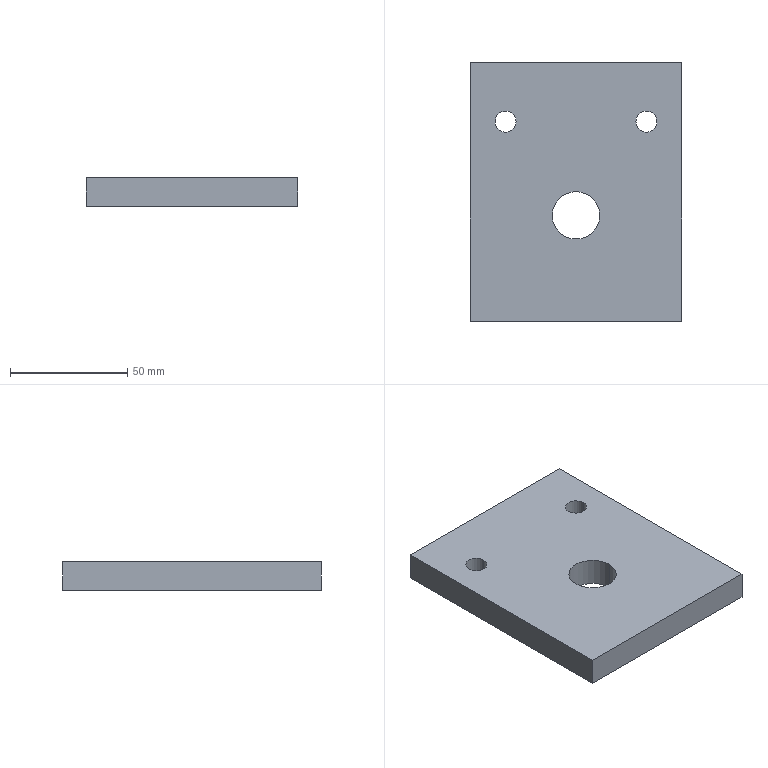Part | SolidWorks | features Extrusion 1, ICE 1 | 1 solid | 12 faces | box 90 x 110 x 12 mm | volume 113427 mm3 | cylinder 6 | plane 6 | commonest cylinder face diameters 9 x4 20.2 x2
STEP:
#1=CARTESIAN_POINT('',(-34.5,30.,-6.));
#2=VERTEX_POINT('',#1);
#3=CARTESIAN_POINT('',(-25.5,30.,-6.));
#4=VERTEX_POINT('',#3);
#5=CARTESIAN_POINT('',(-30.,30.,-6.));
#6=DIRECTION('',(0.,0.,1.));
#7=DIRECTION('',(1.,0.,0.));
#8=AXIS2_PLACEMENT_3D('',#5,#6,#7);
#9=CIRCLE('',#8,4.5);
#10=EDGE_CURVE('',#2,#4,#9,.T.);
#11=ORIENTED_EDGE('',*,*,#10,.F.);
#12=CARTESIAN_POINT('',(-34.5,30.,6.));
#13=VERTEX_POINT('',#12);
#14=CARTESIAN_POINT('',(-34.5,30.,-16.));
#15=DIRECTION('',(0.,0.,1.));
#16=VECTOR('',#15,1000.);
#17=LINE('',#14,#16);
#18=EDGE_CURVE('',#2,#13,#17,.T.);
#19=ORIENTED_EDGE('',*,*,#18,.T.);
#20=CARTESIAN_POINT('',(-25.5,30.,6.));
#21=VERTEX_POINT('',#20);
#22=CARTESIAN_POINT('',(-30.,30.,6.));
#23=DIRECTION('',(0.,0.,1.));
#24=DIRECTION('',(1.,0.,0.));
#25=AXIS2_PLACEMENT_3D('',#22,#23,#24);
#26=CIRCLE('',#25,4.5);
#27=EDGE_CURVE('',#13,#21,#26,.T.);
#28=ORIENTED_EDGE('',*,*,#27,.T.);
#29=CARTESIAN_POINT('',(-25.5,30.,-16.));
#30=DIRECTION('',(0.,0.,1.));
#31=VECTOR('',#30,1000.);
#32=LINE('',#29,#31);
#33=EDGE_CURVE('',#4,#21,#32,.T.);
#34=ORIENTED_EDGE('',*,*,#33,.F.);
#35=EDGE_LOOP('',(#11,#19,#28,#34));
#36=FACE_OUTER_BOUND('',#35,.T.);
#37=CARTESIAN_POINT('',(-30.,30.,-16.));
#38=DIRECTION('',(0.,0.,1.));
#39=DIRECTION('',(1.,0.,0.));
#40=AXIS2_PLACEMENT_3D('',#37,#38,#39);
#41=CYLINDRICAL_SURFACE('',#40,4.5);
#42=ADVANCED_FACE('',(#36),#41,.F.);
#43=CARTESIAN_POINT('',(25.5,30.,-6.));
#44=VERTEX_POINT('',#43);
#45=CARTESIAN_POINT('',(34.5,30.,-6.));
#46=VERTEX_POINT('',#45);
#47=CARTESIAN_POINT('',(30.,30.,-6.));
#48=DIRECTION('',(0.,0.,1.));
#49=DIRECTION('',(1.,0.,0.));
#50=AXIS2_PLACEMENT_3D('',#47,#48,#49);
#51=CIRCLE('',#50,4.5);
#52=EDGE_CURVE('',#44,#46,#51,.T.);
#53=ORIENTED_EDGE('',*,*,#52,.F.);
#54=CARTESIAN_POINT('',(25.5,30.,6.));
#55=VERTEX_POINT('',#54);
#56=CARTESIAN_POINT('',(25.5,30.,-16.));
#57=DIRECTION('',(0.,0.,1.));
#58=VECTOR('',#57,1000.);
#59=LINE('',#56,#58);
#60=EDGE_CURVE('',#44,#55,#59,.T.);
#61=ORIENTED_EDGE('',*,*,#60,.T.);
#62=CARTESIAN_POINT('',(34.5,30.,6.));
#63=VERTEX_POINT('',#62);
#64=CARTESIAN_POINT('',(30.,30.,6.));
#65=DIRECTION('',(0.,0.,1.));
#66=DIRECTION('',(1.,0.,0.));
#67=AXIS2_PLACEMENT_3D('',#64,#65,#66);
#68=CIRCLE('',#67,4.5);
#69=EDGE_CURVE('',#55,#63,#68,.T.);
#70=ORIENTED_EDGE('',*,*,#69,.T.);
#71=CARTESIAN_POINT('',(34.5,30.,-16.));
#72=DIRECTION('',(0.,0.,1.));
#73=VECTOR('',#72,1000.);
#74=LINE('',#71,#73);
#75=EDGE_CURVE('',#46,#63,#74,.T.);
#76=ORIENTED_EDGE('',*,*,#75,.F.);
#77=EDGE_LOOP('',(#53,#61,#70,#76));
#78=FACE_OUTER_BOUND('',#77,.T.);
#79=CARTESIAN_POINT('',(30.,30.,-16.));
#80=DIRECTION('',(0.,0.,1.));
#81=DIRECTION('',(1.,0.,0.));
#82=AXIS2_PLACEMENT_3D('',#79,#80,#81);
#83=CYLINDRICAL_SURFACE('',#82,4.5);
#84=ADVANCED_FACE('',(#78),#83,.F.);
#85=CARTESIAN_POINT('',(-10.1,-10.,-6.));
#86=VERTEX_POINT('',#85);
#87=CARTESIAN_POINT('',(10.1,-10.,-6.));
#88=VERTEX_POINT('',#87);
#89=CARTESIAN_POINT('',(0.,-10.,-6.));
#90=DIRECTION('',(0.,0.,1.));
#91=DIRECTION('',(1.,0.,0.));
#92=AXIS2_PLACEMENT_3D('',#89,#90,#91);
#93=CIRCLE('',#92,10.1);
#94=EDGE_CURVE('',#86,#88,#93,.T.);
#95=ORIENTED_EDGE('',*,*,#94,.F.);
#96=CARTESIAN_POINT('',(-10.1,-10.,6.));
#97=VERTEX_POINT('',#96);
#98=CARTESIAN_POINT('',(-10.1,-10.,-16.));
#99=DIRECTION('',(0.,0.,1.));
#100=VECTOR('',#99,1000.);
#101=LINE('',#98,#100);
#102=EDGE_CURVE('',#86,#97,#101,.T.);
#103=ORIENTED_EDGE('',*,*,#102,.T.);
#104=CARTESIAN_POINT('',(10.1,-10.,6.));
#105=VERTEX_POINT('',#104);
#106=CARTESIAN_POINT('',(0.,-10.,6.));
#107=DIRECTION('',(0.,0.,1.));
#108=DIRECTION('',(1.,0.,0.));
#109=AXIS2_PLACEMENT_3D('',#106,#107,#108);
#110=CIRCLE('',#109,10.1);
#111=EDGE_CURVE('',#97,#105,#110,.T.);
#112=ORIENTED_EDGE('',*,*,#111,.T.);
#113=CARTESIAN_POINT('',(10.1,-10.,-16.));
#114=DIRECTION('',(0.,0.,1.));
#115=VECTOR('',#114,1000.);
#116=LINE('',#113,#115);
#117=EDGE_CURVE('',#88,#105,#116,.T.);
#118=ORIENTED_EDGE('',*,*,#117,.F.);
#119=EDGE_LOOP('',(#95,#103,#112,#118));
#120=FACE_OUTER_BOUND('',#119,.T.);
#121=CARTESIAN_POINT('',(0.,-10.,-16.));
#122=DIRECTION('',(0.,0.,1.));
#123=DIRECTION('',(1.,0.,0.));
#124=AXIS2_PLACEMENT_3D('',#121,#122,#123);
#125=CYLINDRICAL_SURFACE('',#124,10.1);
#126=ADVANCED_FACE('',(#120),#125,.F.);
#127=CARTESIAN_POINT('',(-45.,55.,6.));
#128=VERTEX_POINT('',#127);
#129=CARTESIAN_POINT('',(-45.,-55.,6.));
#130=VERTEX_POINT('',#129);
#131=CARTESIAN_POINT('',(-45.,55.,6.));
#132=DIRECTION('',(0.,-1.,0.));
#133=VECTOR('',#132,1000.);
#134=LINE('',#131,#133);
#135=EDGE_CURVE('',#128,#130,#134,.T.);
#136=ORIENTED_EDGE('',*,*,#135,.F.);
#137=CARTESIAN_POINT('',(-45.,55.,-6.));
#138=VERTEX_POINT('',#137);
#139=CARTESIAN_POINT('',(-45.,55.,-6.));
#140=DIRECTION('',(0.,0.,1.));
#141=VECTOR('',#140,1000.);
#142=LINE('',#139,#141);
#143=EDGE_CURVE('',#138,#128,#142,.T.);
#144=ORIENTED_EDGE('',*,*,#143,.F.);
#145=CARTESIAN_POINT('',(-45.,-55.,-6.));
#146=VERTEX_POINT('',#145);
#147=CARTESIAN_POINT('',(-45.,55.,-6.));
#148=DIRECTION('',(0.,-1.,0.));
#149=VECTOR('',#148,1000.);
#150=LINE('',#147,#149);
#151=EDGE_CURVE('',#138,#146,#150,.T.);
#152=ORIENTED_EDGE('',*,*,#151,.T.);
#153=CARTESIAN_POINT('',(-45.,-55.,-6.));
#154=DIRECTION('',(0.,0.,1.));
#155=VECTOR('',#154,1000.);
#156=LINE('',#153,#155);
#157=EDGE_CURVE('',#146,#130,#156,.T.);
#158=ORIENTED_EDGE('',*,*,#157,.T.);
#159=EDGE_LOOP('',(#136,#144,#152,#158));
#160=FACE_OUTER_BOUND('',#159,.T.);
#161=CARTESIAN_POINT('',(-45.,55.,-6.));
#162=DIRECTION('',(-1.,0.,0.));
#163=DIRECTION('',(0.,0.,1.));
#164=AXIS2_PLACEMENT_3D('',#161,#162,#163);
#165=PLANE('',#164);
#166=ADVANCED_FACE('',(#160),#165,.T.);
#167=CARTESIAN_POINT('',(45.,55.,6.));
#168=VERTEX_POINT('',#167);
#169=CARTESIAN_POINT('',(45.,55.,6.));
#170=DIRECTION('',(-1.,0.,0.));
#171=VECTOR('',#170,1000.);
#172=LINE('',#169,#171);
#173=EDGE_CURVE('',#168,#128,#172,.T.);
#174=ORIENTED_EDGE('',*,*,#173,.F.);
#175=CARTESIAN_POINT('',(45.,55.,-6.));
#176=VERTEX_POINT('',#175);
#177=CARTESIAN_POINT('',(45.,55.,-6.));
#178=DIRECTION('',(0.,0.,1.));
#179=VECTOR('',#178,1000.);
#180=LINE('',#177,#179);
#181=EDGE_CURVE('',#176,#168,#180,.T.);
#182=ORIENTED_EDGE('',*,*,#181,.F.);
#183=CARTESIAN_POINT('',(45.,55.,-6.));
#184=DIRECTION('',(-1.,0.,0.));
#185=VECTOR('',#184,1000.);
#186=LINE('',#183,#185);
#187=EDGE_CURVE('',#176,#138,#186,.T.);
#188=ORIENTED_EDGE('',*,*,#187,.T.);
#189=ORIENTED_EDGE('',*,*,#143,.T.);
#190=EDGE_LOOP('',(#174,#182,#188,#189));
#191=FACE_OUTER_BOUND('',#190,.T.);
#192=CARTESIAN_POINT('',(45.,55.,-6.));
#193=DIRECTION('',(0.,1.,0.));
#194=DIRECTION('',(0.,0.,1.));
#195=AXIS2_PLACEMENT_3D('',#192,#193,#194);
#196=PLANE('',#195);
#197=ADVANCED_FACE('',(#191),#196,.T.);
#198=CARTESIAN_POINT('',(45.,-55.,6.));
#199=VERTEX_POINT('',#198);
#200=CARTESIAN_POINT('',(45.,-55.,6.));
#201=DIRECTION('',(0.,1.,0.));
#202=VECTOR('',#201,1000.);
#203=LINE('',#200,#202);
#204=EDGE_CURVE('',#199,#168,#203,.T.);
#205=ORIENTED_EDGE('',*,*,#204,.F.);
#206=CARTESIAN_POINT('',(45.,-55.,-6.));
#207=VERTEX_POINT('',#206);
#208=CARTESIAN_POINT('',(45.,-55.,-6.));
#209=DIRECTION('',(0.,0.,1.));
#210=VECTOR('',#209,1000.);
#211=LINE('',#208,#210);
#212=EDGE_CURVE('',#207,#199,#211,.T.);
#213=ORIENTED_EDGE('',*,*,#212,.F.);
#214=CARTESIAN_POINT('',(45.,-55.,-6.));
#215=DIRECTION('',(0.,1.,0.));
#216=VECTOR('',#215,1000.);
#217=LINE('',#214,#216);
#218=EDGE_CURVE('',#207,#176,#217,.T.);
#219=ORIENTED_EDGE('',*,*,#218,.T.);
#220=ORIENTED_EDGE('',*,*,#181,.T.);
#221=EDGE_LOOP('',(#205,#213,#219,#220));
#222=FACE_OUTER_BOUND('',#221,.T.);
#223=CARTESIAN_POINT('',(45.,-55.,-6.));
#224=DIRECTION('',(1.,0.,0.));
#225=DIRECTION('',(0.,0.,-1.));
#226=AXIS2_PLACEMENT_3D('',#223,#224,#225);
#227=PLANE('',#226);
#228=ADVANCED_FACE('',(#222),#227,.T.);
#229=CARTESIAN_POINT('',(-45.,-55.,6.));
#230=DIRECTION('',(1.,0.,0.));
#231=VECTOR('',#230,1000.);
#232=LINE('',#229,#231);
#233=EDGE_CURVE('',#130,#199,#232,.T.);
#234=ORIENTED_EDGE('',*,*,#233,.F.);
#235=ORIENTED_EDGE('',*,*,#157,.F.);
#236=CARTESIAN_POINT('',(-45.,-55.,-6.));
#237=DIRECTION('',(1.,0.,0.));
#238=VECTOR('',#237,1000.);
#239=LINE('',#236,#238);
#240=EDGE_CURVE('',#146,#207,#239,.T.);
#241=ORIENTED_EDGE('',*,*,#240,.T.);
#242=ORIENTED_EDGE('',*,*,#212,.T.);
#243=EDGE_LOOP('',(#234,#235,#241,#242));
#244=FACE_OUTER_BOUND('',#243,.T.);
#245=CARTESIAN_POINT('',(-45.,-55.,-6.));
#246=DIRECTION('',(0.,-1.,0.));
#247=DIRECTION('',(0.,0.,-1.));
#248=AXIS2_PLACEMENT_3D('',#245,#246,#247);
#249=PLANE('',#248);
#250=ADVANCED_FACE('',(#244),#249,.T.);
#251=CARTESIAN_POINT('',(-30.,30.,-6.));
#252=DIRECTION('',(0.,0.,1.));
#253=DIRECTION('',(1.,0.,0.));
#254=AXIS2_PLACEMENT_3D('',#251,#252,#253);
#255=CIRCLE('',#254,4.5);
#256=EDGE_CURVE('',#4,#2,#255,.T.);
#257=ORIENTED_EDGE('',*,*,#256,.T.);
#258=ORIENTED_EDGE('',*,*,#10,.T.);
#259=EDGE_LOOP('',(#257,#258));
#260=FACE_BOUND('',#259,.T.);
#261=CARTESIAN_POINT('',(30.,30.,-6.));
#262=DIRECTION('',(0.,0.,1.));
#263=DIRECTION('',(1.,0.,0.));
#264=AXIS2_PLACEMENT_3D('',#261,#262,#263);
#265=CIRCLE('',#264,4.5);
#266=EDGE_CURVE('',#46,#44,#265,.T.);
#267=ORIENTED_EDGE('',*,*,#266,.T.);
#268=ORIENTED_EDGE('',*,*,#52,.T.);
#269=EDGE_LOOP('',(#267,#268));
#270=FACE_BOUND('',#269,.T.);
#271=CARTESIAN_POINT('',(0.,-10.,-6.));
#272=DIRECTION('',(0.,0.,1.));
#273=DIRECTION('',(1.,0.,0.));
#274=AXIS2_PLACEMENT_3D('',#271,#272,#273);
#275=CIRCLE('',#274,10.1);
#276=EDGE_CURVE('',#88,#86,#275,.T.);
#277=ORIENTED_EDGE('',*,*,#276,.T.);
#278=ORIENTED_EDGE('',*,*,#94,.T.);
#279=EDGE_LOOP('',(#277,#278));
#280=FACE_BOUND('',#279,.T.);
#281=ORIENTED_EDGE('',*,*,#151,.F.);
#282=ORIENTED_EDGE('',*,*,#187,.F.);
#283=ORIENTED_EDGE('',*,*,#218,.F.);
#284=ORIENTED_EDGE('',*,*,#240,.F.);
#285=EDGE_LOOP('',(#281,#282,#283,#284));
#286=FACE_OUTER_BOUND('',#285,.T.);
#287=CARTESIAN_POINT('',(0.,0.,-6.));
#288=DIRECTION('',(0.,0.,1.));
#289=DIRECTION('',(1.,0.,0.));
#290=AXIS2_PLACEMENT_3D('',#287,#288,#289);
#291=PLANE('',#290);
#292=ADVANCED_FACE('',(#260,#270,#280,#286),#291,.F.);
#293=CARTESIAN_POINT('',(-30.,30.,6.));
#294=DIRECTION('',(0.,0.,1.));
#295=DIRECTION('',(1.,0.,0.));
#296=AXIS2_PLACEMENT_3D('',#293,#294,#295);
#297=CIRCLE('',#296,4.5);
#298=EDGE_CURVE('',#21,#13,#297,.T.);
#299=ORIENTED_EDGE('',*,*,#298,.F.);
#300=ORIENTED_EDGE('',*,*,#27,.F.);
#301=EDGE_LOOP('',(#299,#300));
#302=FACE_BOUND('',#301,.T.);
#303=CARTESIAN_POINT('',(30.,30.,6.));
#304=DIRECTION('',(0.,0.,1.));
#305=DIRECTION('',(1.,0.,0.));
#306=AXIS2_PLACEMENT_3D('',#303,#304,#305);
#307=CIRCLE('',#306,4.5);
#308=EDGE_CURVE('',#63,#55,#307,.T.);
#309=ORIENTED_EDGE('',*,*,#308,.F.);
#310=ORIENTED_EDGE('',*,*,#69,.F.);
#311=EDGE_LOOP('',(#309,#310));
#312=FACE_BOUND('',#311,.T.);
#313=CARTESIAN_POINT('',(0.,-10.,6.));
#314=DIRECTION('',(0.,0.,1.));
#315=DIRECTION('',(1.,0.,0.));
#316=AXIS2_PLACEMENT_3D('',#313,#314,#315);
#317=CIRCLE('',#316,10.1);
#318=EDGE_CURVE('',#105,#97,#317,.T.);
#319=ORIENTED_EDGE('',*,*,#318,.F.);
#320=ORIENTED_EDGE('',*,*,#111,.F.);
#321=EDGE_LOOP('',(#319,#320));
#322=FACE_BOUND('',#321,.T.);
#323=ORIENTED_EDGE('',*,*,#135,.T.);
#324=ORIENTED_EDGE('',*,*,#233,.T.);
#325=ORIENTED_EDGE('',*,*,#204,.T.);
#326=ORIENTED_EDGE('',*,*,#173,.T.);
#327=EDGE_LOOP('',(#323,#324,#325,#326));
#328=FACE_OUTER_BOUND('',#327,.T.);
#329=CARTESIAN_POINT('',(0.,0.,6.));
#330=DIRECTION('',(0.,0.,1.));
#331=DIRECTION('',(1.,0.,0.));
#332=AXIS2_PLACEMENT_3D('',#329,#330,#331);
#333=PLANE('',#332);
#334=ADVANCED_FACE('',(#302,#312,#322,#328),#333,.T.);
#335=ORIENTED_EDGE('',*,*,#102,.F.);
#336=ORIENTED_EDGE('',*,*,#276,.F.);
#337=ORIENTED_EDGE('',*,*,#117,.T.);
#338=ORIENTED_EDGE('',*,*,#318,.T.);
#339=EDGE_LOOP('',(#335,#336,#337,#338));
#340=FACE_OUTER_BOUND('',#339,.T.);
#341=CARTESIAN_POINT('',(0.,-10.,-16.));
#342=DIRECTION('',(0.,0.,1.));
#343=DIRECTION('',(1.,0.,0.));
#344=AXIS2_PLACEMENT_3D('',#341,#342,#343);
#345=CYLINDRICAL_SURFACE('',#344,10.1);
#346=ADVANCED_FACE('',(#340),#345,.F.);
#347=ORIENTED_EDGE('',*,*,#60,.F.);
#348=ORIENTED_EDGE('',*,*,#266,.F.);
#349=ORIENTED_EDGE('',*,*,#75,.T.);
#350=ORIENTED_EDGE('',*,*,#308,.T.);
#351=EDGE_LOOP('',(#347,#348,#349,#350));
#352=FACE_OUTER_BOUND('',#351,.T.);
#353=CARTESIAN_POINT('',(30.,30.,-16.));
#354=DIRECTION('',(0.,0.,1.));
#355=DIRECTION('',(1.,0.,0.));
#356=AXIS2_PLACEMENT_3D('',#353,#354,#355);
#357=CYLINDRICAL_SURFACE('',#356,4.5);
#358=ADVANCED_FACE('',(#352),#357,.F.);
#359=ORIENTED_EDGE('',*,*,#18,.F.);
#360=ORIENTED_EDGE('',*,*,#256,.F.);
#361=ORIENTED_EDGE('',*,*,#33,.T.);
#362=ORIENTED_EDGE('',*,*,#298,.T.);
#363=EDGE_LOOP('',(#359,#360,#361,#362));
#364=FACE_OUTER_BOUND('',#363,.T.);
#365=CARTESIAN_POINT('',(-30.,30.,-16.));
#366=DIRECTION('',(0.,0.,1.));
#367=DIRECTION('',(1.,0.,0.));
#368=AXIS2_PLACEMENT_3D('',#365,#366,#367);
#369=CYLINDRICAL_SURFACE('',#368,4.5);
#370=ADVANCED_FACE('',(#364),#369,.F.);
#371=CLOSED_SHELL('',(#42,#84,#126,#166,#197,#228,#250,#292,#334,#346,#358,#370));
#372=MANIFOLD_SOLID_BREP('',#371);
#373=CARTESIAN_POINT('',(0.,0.,0.));
#374=DIRECTION('',(0.,0.,1.));
#375=DIRECTION('',(1.,0.,0.));
#376=AXIS2_PLACEMENT_3D('',#373,#374,#375);
#377=(LENGTH_UNIT()NAMED_UNIT(*)SI_UNIT(.MILLI.,.METRE.));
#378=UNCERTAINTY_MEASURE_WITH_UNIT(LENGTH_MEASURE(0.00001),#377,'','');
#379=(NAMED_UNIT(*)PLANE_ANGLE_UNIT()SI_UNIT($,.RADIAN.));
#380=(NAMED_UNIT(*)SI_UNIT($,.STERADIAN.)SOLID_ANGLE_UNIT());
#381=(GEOMETRIC_REPRESENTATION_CONTEXT(3)GLOBAL_UNCERTAINTY_ASSIGNED_CONTEXT((#378))GLOBAL_UNIT_ASSIGNED_CONTEXT((#377,#379,#380))REPRESENTATION_CONTEXT('',''));
#382=ADVANCED_BREP_SHAPE_REPRESENTATION('',(#372,#376),#381);